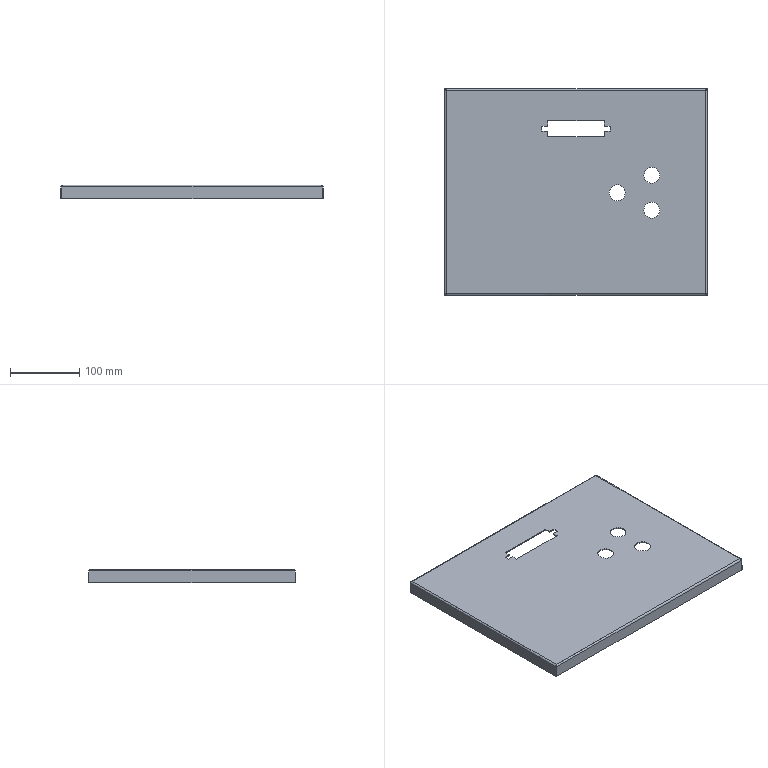Part | SolidWorks | features Cut 3, CornerFeat 1, EdgeFlange 1, FlatPattern 1, ICE 1, LPattern 1, LibraryFeature 1, SMBaseFlange 1, SheetMetal 1 | 1 solid | 56 faces | box 378.8 x 297.75 x 19.5 mm | volume 199133 mm3 | plane 34 | cylinder 14 | spline 8 | commonest cylinder face diameters 23 x6 2 x4 5 x4